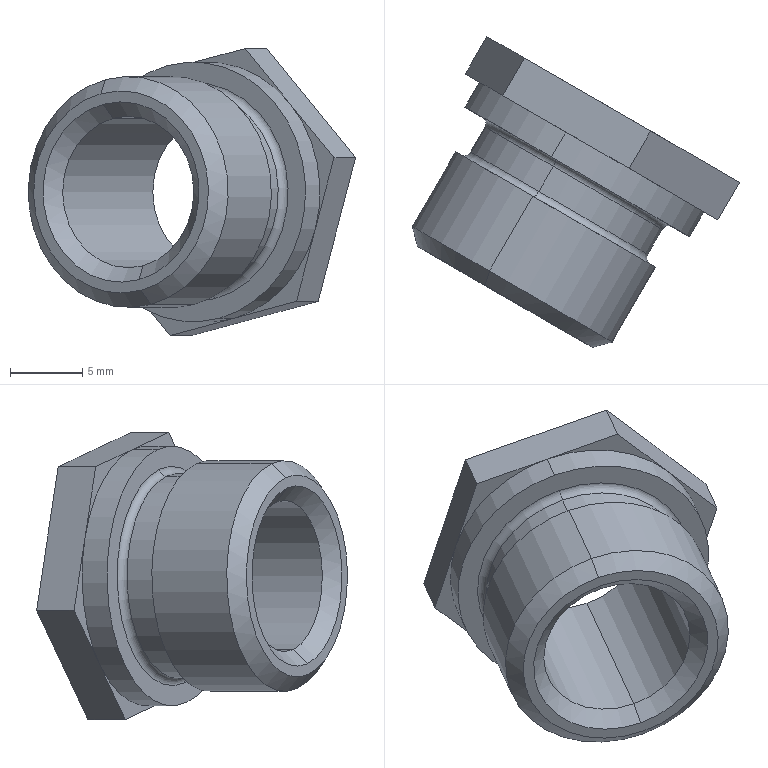Part | SolidWorks | features BaseBody 1 | 1 solid | 34 faces | box 22.69 x 21.549 x 19.899 mm | volume 1857 mm3 | plane 16 | cylinder 8 | cone 6 | torus 4 | commonest cylinder face diameters 10.5 x2 14.2 x2 16 x2 18 x2
STEP:
#1=CARTESIAN_POINT('',(323.84,252.406,-5.111));
#2=VERTEX_POINT('',#1);
#3=CARTESIAN_POINT('',(321.76,253.606,5.111));
#4=VERTEX_POINT('',#3);
#5=CARTESIAN_POINT('',(322.8,253.006,0.));
#6=DIRECTION('',(-0.5,-0.866,0.));
#7=DIRECTION('',(-0.198,0.1143,0.9735));
#8=AXIS2_PLACEMENT_3D('',#5,#6,#7);
#9=CIRCLE('',#8,5.25);
#10=EDGE_CURVE('',#2,#4,#9,.T.);
#11=ORIENTED_EDGE('',*,*,#10,.F.);
#12=CARTESIAN_POINT('',(323.538,251.425,-6.084));
#13=VERTEX_POINT('',#12);
#14=CARTESIAN_POINT('',(323.538,251.425,-6.084));
#15=DIRECTION('',(-0.2135,-0.6932,-0.6884));
#16=VECTOR('',#15,1000.);
#17=LINE('',#14,#16);
#18=EDGE_CURVE('',#2,#13,#17,.T.);
#19=ORIENTED_EDGE('',*,*,#18,.T.);
#20=CARTESIAN_POINT('',(321.062,252.854,6.084));
#21=VERTEX_POINT('',#20);
#22=CARTESIAN_POINT('',(322.3,252.14,0.));
#23=DIRECTION('',(0.5,0.866,0.));
#24=DIRECTION('',(-0.198,0.1143,0.9735));
#25=AXIS2_PLACEMENT_3D('',#22,#23,#24);
#26=CIRCLE('',#25,6.25);
#27=EDGE_CURVE('',#21,#13,#26,.T.);
#28=ORIENTED_EDGE('',*,*,#27,.F.);
#29=CARTESIAN_POINT('',(321.062,252.854,6.084));
#30=DIRECTION('',(-0.4936,-0.5315,0.6884));
#31=VECTOR('',#30,1000.);
#32=LINE('',#29,#31);
#33=EDGE_CURVE('',#4,#21,#32,.T.);
#34=ORIENTED_EDGE('',*,*,#33,.F.);
#35=EDGE_LOOP('',(#11,#19,#28,#34));
#36=FACE_OUTER_BOUND('',#35,.T.);
#37=CARTESIAN_POINT('',(322.3,252.14,0.));
#38=DIRECTION('',(-0.5,-0.866,0.));
#39=DIRECTION('',(-0.198,0.1143,0.9735));
#40=AXIS2_PLACEMENT_3D('',#37,#38,#39);
#41=CONICAL_SURFACE('',#40,6.25,0.7854);
#42=ADVANCED_FACE('',(#36),#41,.F.);
#43=CARTESIAN_POINT('',(328.01,264.431,5.111));
#44=VERTEX_POINT('',#43);
#45=CARTESIAN_POINT('',(330.09,263.231,-5.111));
#46=VERTEX_POINT('',#45);
#47=CARTESIAN_POINT('',(329.05,263.831,0.));
#48=DIRECTION('',(0.5,0.866,0.));
#49=DIRECTION('',(0.198,-0.1143,-0.9735));
#50=AXIS2_PLACEMENT_3D('',#47,#48,#49);
#51=CIRCLE('',#50,5.25);
#52=EDGE_CURVE('',#44,#46,#51,.T.);
#53=ORIENTED_EDGE('',*,*,#52,.F.);
#54=CARTESIAN_POINT('',(328.463,265.902,6.571));
#55=VERTEX_POINT('',#54);
#56=CARTESIAN_POINT('',(328.01,264.431,5.111));
#57=DIRECTION('',(0.2135,0.6932,0.6884));
#58=VECTOR('',#57,1000.);
#59=LINE('',#56,#58);
#60=EDGE_CURVE('',#44,#55,#59,.T.);
#61=ORIENTED_EDGE('',*,*,#60,.T.);
#62=CARTESIAN_POINT('',(331.137,264.358,-6.571));
#63=VERTEX_POINT('',#62);
#64=CARTESIAN_POINT('',(329.8,265.13,0.));
#65=DIRECTION('',(-0.5,-0.866,0.));
#66=DIRECTION('',(0.198,-0.1143,-0.9735));
#67=AXIS2_PLACEMENT_3D('',#64,#65,#66);
#68=CIRCLE('',#67,6.75);
#69=EDGE_CURVE('',#63,#55,#68,.T.);
#70=ORIENTED_EDGE('',*,*,#69,.F.);
#71=CARTESIAN_POINT('',(330.09,263.231,-5.111));
#72=DIRECTION('',(0.4936,0.5315,-0.6884));
#73=VECTOR('',#72,1000.);
#74=LINE('',#71,#73);
#75=EDGE_CURVE('',#46,#63,#74,.T.);
#76=ORIENTED_EDGE('',*,*,#75,.F.);
#77=EDGE_LOOP('',(#53,#61,#70,#76));
#78=FACE_OUTER_BOUND('',#77,.T.);
#79=CARTESIAN_POINT('',(329.05,263.831,0.));
#80=DIRECTION('',(0.5,0.866,0.));
#81=DIRECTION('',(0.198,-0.1143,-0.9735));
#82=AXIS2_PLACEMENT_3D('',#79,#80,#81);
#83=CONICAL_SURFACE('',#82,5.25,0.7854);
#84=ADVANCED_FACE('',(#78),#83,.F.);
#85=ORIENTED_EDGE('',*,*,#10,.T.);
#86=CARTESIAN_POINT('',(321.26,252.74,5.111));
#87=DIRECTION('',(0.5,0.866,0.));
#88=VECTOR('',#87,1000.);
#89=LINE('',#86,#88);
#90=EDGE_CURVE('',#4,#44,#89,.T.);
#91=ORIENTED_EDGE('',*,*,#90,.T.);
#92=ORIENTED_EDGE('',*,*,#52,.T.);
#93=CARTESIAN_POINT('',(323.34,251.54,-5.111));
#94=DIRECTION('',(0.5,0.866,0.));
#95=VECTOR('',#94,1000.);
#96=LINE('',#93,#95);
#97=EDGE_CURVE('',#2,#46,#96,.T.);
#98=ORIENTED_EDGE('',*,*,#97,.F.);
#99=EDGE_LOOP('',(#85,#91,#92,#98));
#100=FACE_OUTER_BOUND('',#99,.T.);
#101=CARTESIAN_POINT('',(322.3,252.14,0.));
#102=DIRECTION('',(0.5,0.866,0.));
#103=DIRECTION('',(0.198,-0.1143,-0.9735));
#104=AXIS2_PLACEMENT_3D('',#101,#102,#103);
#105=CYLINDRICAL_SURFACE('',#104,5.25);
#106=ADVANCED_FACE('',(#100),#105,.F.);
#107=CARTESIAN_POINT('',(327.305,257.333,-7.399));
#108=VERTEX_POINT('',#107);
#109=CARTESIAN_POINT('',(324.295,259.071,7.399));
#110=VERTEX_POINT('',#109);
#111=CARTESIAN_POINT('',(325.8,258.202,0.));
#112=DIRECTION('',(-0.5,-0.866,0.));
#113=DIRECTION('',(-0.198,0.1143,0.9735));
#114=AXIS2_PLACEMENT_3D('',#111,#112,#113);
#115=CIRCLE('',#114,7.6);
#116=EDGE_CURVE('',#108,#110,#115,.T.);
#117=ORIENTED_EDGE('',*,*,#116,.F.);
#118=CARTESIAN_POINT('',(327.456,257.823,-6.912));
#119=VERTEX_POINT('',#118);
#120=CARTESIAN_POINT('',(327.555,257.766,-7.399));
#121=DIRECTION('',(-0.8431,0.4868,-0.2286));
#122=DIRECTION('',(-0.5,-0.866,0.));
#123=AXIS2_PLACEMENT_3D('',#120,#121,#122);
#124=CIRCLE('',#123,0.5);
#125=EDGE_CURVE('',#108,#119,#124,.T.);
#126=ORIENTED_EDGE('',*,*,#125,.T.);
#127=CARTESIAN_POINT('',(324.644,259.447,6.912));
#128=VERTEX_POINT('',#127);
#129=CARTESIAN_POINT('',(326.05,258.635,0.));
#130=DIRECTION('',(0.5,0.866,0.));
#131=DIRECTION('',(-0.198,0.1143,0.9735));
#132=AXIS2_PLACEMENT_3D('',#129,#130,#131);
#133=CIRCLE('',#132,7.1);
#134=EDGE_CURVE('',#128,#119,#133,.T.);
#135=ORIENTED_EDGE('',*,*,#134,.F.);
#136=CARTESIAN_POINT('',(324.545,259.504,7.399));
#137=DIRECTION('',(0.8431,-0.4868,0.2286));
#138=DIRECTION('',(0.5,0.866,0.));
#139=AXIS2_PLACEMENT_3D('',#136,#137,#138);
#140=CIRCLE('',#139,0.5);
#141=EDGE_CURVE('',#110,#128,#140,.T.);
#142=ORIENTED_EDGE('',*,*,#141,.F.);
#143=EDGE_LOOP('',(#117,#126,#135,#142));
#144=FACE_OUTER_BOUND('',#143,.T.);
#145=CARTESIAN_POINT('',(326.05,258.635,0.));
#146=DIRECTION('',(-0.5,-0.866,0.));
#147=DIRECTION('',(-0.198,0.1143,0.9735));
#148=AXIS2_PLACEMENT_3D('',#145,#146,#147);
#149=TOROIDAL_SURFACE('',#148,7.6,0.5);
#150=ADVANCED_FACE('',(#144),#149,.F.);
#151=CARTESIAN_POINT('',(328.456,259.555,-6.912));
#152=VERTEX_POINT('',#151);
#153=CARTESIAN_POINT('',(325.644,261.179,6.912));
#154=VERTEX_POINT('',#153);
#155=CARTESIAN_POINT('',(327.05,260.367,0.));
#156=DIRECTION('',(-0.5,-0.866,0.));
#157=DIRECTION('',(-0.198,0.1143,0.9735));
#158=AXIS2_PLACEMENT_3D('',#155,#156,#157);
#159=CIRCLE('',#158,7.1);
#160=EDGE_CURVE('',#152,#154,#159,.T.);
#161=ORIENTED_EDGE('',*,*,#160,.F.);
#162=CARTESIAN_POINT('',(328.805,259.931,-7.399));
#163=VERTEX_POINT('',#162);
#164=CARTESIAN_POINT('',(328.555,259.498,-7.399));
#165=DIRECTION('',(-0.8431,0.4868,-0.2286));
#166=DIRECTION('',(-0.5,-0.866,0.));
#167=AXIS2_PLACEMENT_3D('',#164,#165,#166);
#168=CIRCLE('',#167,0.5);
#169=EDGE_CURVE('',#152,#163,#168,.T.);
#170=ORIENTED_EDGE('',*,*,#169,.T.);
#171=CARTESIAN_POINT('',(325.795,261.669,7.399));
#172=VERTEX_POINT('',#171);
#173=CARTESIAN_POINT('',(327.3,260.8,0.));
#174=DIRECTION('',(0.5,0.866,0.));
#175=DIRECTION('',(-0.198,0.1143,0.9735));
#176=AXIS2_PLACEMENT_3D('',#173,#174,#175);
#177=CIRCLE('',#176,7.6);
#178=EDGE_CURVE('',#172,#163,#177,.T.);
#179=ORIENTED_EDGE('',*,*,#178,.F.);
#180=CARTESIAN_POINT('',(325.545,261.236,7.399));
#181=DIRECTION('',(0.8431,-0.4868,0.2286));
#182=DIRECTION('',(0.5,0.866,0.));
#183=AXIS2_PLACEMENT_3D('',#180,#181,#182);
#184=CIRCLE('',#183,0.5);
#185=EDGE_CURVE('',#154,#172,#184,.T.);
#186=ORIENTED_EDGE('',*,*,#185,.F.);
#187=EDGE_LOOP('',(#161,#170,#179,#186));
#188=FACE_OUTER_BOUND('',#187,.T.);
#189=CARTESIAN_POINT('',(327.05,260.367,0.));
#190=DIRECTION('',(-0.5,-0.866,0.));
#191=DIRECTION('',(-0.198,0.1143,0.9735));
#192=AXIS2_PLACEMENT_3D('',#189,#190,#191);
#193=TOROIDAL_SURFACE('',#192,7.6,0.5);
#194=ADVANCED_FACE('',(#188),#193,.F.);
#195=CARTESIAN_POINT('',(320.914,252.94,6.815));
#196=VERTEX_POINT('',#195);
#197=CARTESIAN_POINT('',(323.686,251.34,-6.815));
#198=VERTEX_POINT('',#197);
#199=CARTESIAN_POINT('',(322.3,252.14,0.));
#200=DIRECTION('',(-0.5,-0.866,0.));
#201=DIRECTION('',(-0.198,0.1143,0.9735));
#202=AXIS2_PLACEMENT_3D('',#199,#200,#201);
#203=CIRCLE('',#202,7.);
#204=EDGE_CURVE('',#196,#198,#203,.T.);
#205=ORIENTED_EDGE('',*,*,#204,.F.);
#206=CARTESIAN_POINT('',(321.216,253.92,7.788));
#207=VERTEX_POINT('',#206);
#208=CARTESIAN_POINT('',(320.914,252.94,6.815));
#209=DIRECTION('',(0.2135,0.6932,0.6884));
#210=VECTOR('',#209,1000.);
#211=LINE('',#208,#210);
#212=EDGE_CURVE('',#196,#207,#211,.T.);
#213=ORIENTED_EDGE('',*,*,#212,.T.);
#214=CARTESIAN_POINT('',(324.384,252.091,-7.788));
#215=VERTEX_POINT('',#214);
#216=CARTESIAN_POINT('',(322.8,253.006,0.));
#217=DIRECTION('',(0.5,0.866,0.));
#218=DIRECTION('',(-0.198,0.1143,0.9735));
#219=AXIS2_PLACEMENT_3D('',#216,#217,#218);
#220=CIRCLE('',#219,8.);
#221=EDGE_CURVE('',#215,#207,#220,.T.);
#222=ORIENTED_EDGE('',*,*,#221,.F.);
#223=CARTESIAN_POINT('',(323.686,251.34,-6.815));
#224=DIRECTION('',(0.4936,0.5315,-0.6884));
#225=VECTOR('',#224,1000.);
#226=LINE('',#223,#225);
#227=EDGE_CURVE('',#198,#215,#226,.T.);
#228=ORIENTED_EDGE('',*,*,#227,.F.);
#229=EDGE_LOOP('',(#205,#213,#222,#228));
#230=FACE_OUTER_BOUND('',#229,.T.);
#231=CARTESIAN_POINT('',(322.3,252.14,0.));
#232=DIRECTION('',(0.5,0.866,0.));
#233=DIRECTION('',(0.198,-0.1143,-0.9735));
#234=AXIS2_PLACEMENT_3D('',#231,#232,#233);
#235=CONICAL_SURFACE('',#234,7.,0.7854);
#236=ADVANCED_FACE('',(#230),#235,.T.);
#237=ORIENTED_EDGE('',*,*,#221,.T.);
#238=CARTESIAN_POINT('',(324.216,259.116,7.788));
#239=VERTEX_POINT('',#238);
#240=CARTESIAN_POINT('',(306.402,228.262,7.788));
#241=DIRECTION('',(0.5,0.866,0.));
#242=VECTOR('',#241,1000.);
#243=LINE('',#240,#242);
#244=EDGE_CURVE('',#207,#239,#243,.T.);
#245=ORIENTED_EDGE('',*,*,#244,.T.);
#246=CARTESIAN_POINT('',(327.384,257.287,-7.788));
#247=VERTEX_POINT('',#246);
#248=CARTESIAN_POINT('',(325.8,258.202,0.));
#249=DIRECTION('',(-0.5,-0.866,0.));
#250=DIRECTION('',(-0.198,0.1143,0.9735));
#251=AXIS2_PLACEMENT_3D('',#248,#249,#250);
#252=CIRCLE('',#251,8.);
#253=EDGE_CURVE('',#239,#247,#252,.T.);
#254=ORIENTED_EDGE('',*,*,#253,.T.);
#255=CARTESIAN_POINT('',(309.57,226.433,-7.788));
#256=DIRECTION('',(0.5,0.866,0.));
#257=VECTOR('',#256,1000.);
#258=LINE('',#255,#257);
#259=EDGE_CURVE('',#215,#247,#258,.T.);
#260=ORIENTED_EDGE('',*,*,#259,.F.);
#261=EDGE_LOOP('',(#237,#245,#254,#260));
#262=FACE_OUTER_BOUND('',#261,.T.);
#263=CARTESIAN_POINT('',(307.986,227.348,0.));
#264=DIRECTION('',(0.5,0.866,0.));
#265=DIRECTION('',(0.198,-0.1143,-0.9735));
#266=AXIS2_PLACEMENT_3D('',#263,#264,#265);
#267=CYLINDRICAL_SURFACE('',#266,8.);
#268=ADVANCED_FACE('',(#262),#267,.T.);
#269=CARTESIAN_POINT('',(326.05,258.635,0.));
#270=DIRECTION('',(0.5,0.866,0.));
#271=DIRECTION('',(-0.198,0.1143,0.9735));
#272=AXIS2_PLACEMENT_3D('',#269,#270,#271);
#273=CIRCLE('',#272,7.1);
#274=EDGE_CURVE('',#119,#128,#273,.T.);
#275=ORIENTED_EDGE('',*,*,#274,.T.);
#276=CARTESIAN_POINT('',(324.394,259.014,6.912));
#277=DIRECTION('',(0.5,0.866,0.));
#278=VECTOR('',#277,1000.);
#279=LINE('',#276,#278);
#280=EDGE_CURVE('',#128,#154,#279,.T.);
#281=ORIENTED_EDGE('',*,*,#280,.T.);
#282=CARTESIAN_POINT('',(327.05,260.367,0.));
#283=DIRECTION('',(-0.5,-0.866,0.));
#284=DIRECTION('',(-0.198,0.1143,0.9735));
#285=AXIS2_PLACEMENT_3D('',#282,#283,#284);
#286=CIRCLE('',#285,7.1);
#287=EDGE_CURVE('',#154,#152,#286,.T.);
#288=ORIENTED_EDGE('',*,*,#287,.T.);
#289=CARTESIAN_POINT('',(327.206,257.39,-6.912));
#290=DIRECTION('',(0.5,0.866,0.));
#291=VECTOR('',#290,1000.);
#292=LINE('',#289,#291);
#293=EDGE_CURVE('',#119,#152,#292,.T.);
#294=ORIENTED_EDGE('',*,*,#293,.F.);
#295=EDGE_LOOP('',(#275,#281,#288,#294));
#296=FACE_OUTER_BOUND('',#295,.T.);
#297=CARTESIAN_POINT('',(325.8,258.202,0.));
#298=DIRECTION('',(0.5,0.866,0.));
#299=DIRECTION('',(0.198,-0.1143,-0.9735));
#300=AXIS2_PLACEMENT_3D('',#297,#298,#299);
#301=CYLINDRICAL_SURFACE('',#300,7.1);
#302=ADVANCED_FACE('',(#296),#301,.T.);
#303=CARTESIAN_POINT('',(325.518,261.829,8.762));
#304=VERTEX_POINT('',#303);
#305=CARTESIAN_POINT('',(329.082,259.771,-8.762));
#306=VERTEX_POINT('',#305);
#307=CARTESIAN_POINT('',(327.3,260.8,0.));
#308=DIRECTION('',(-0.5,-0.866,0.));
#309=DIRECTION('',(-0.198,0.1143,0.9735));
#310=AXIS2_PLACEMENT_3D('',#307,#308,#309);
#311=CIRCLE('',#310,9.);
#312=EDGE_CURVE('',#304,#306,#311,.T.);
#313=ORIENTED_EDGE('',*,*,#312,.F.);
#314=CARTESIAN_POINT('',(326.518,263.561,8.762));
#315=VERTEX_POINT('',#314);
#316=CARTESIAN_POINT('',(325.518,261.829,8.762));
#317=DIRECTION('',(0.5,0.866,0.));
#318=VECTOR('',#317,1000.);
#319=LINE('',#316,#318);
#320=EDGE_CURVE('',#304,#315,#319,.T.);
#321=ORIENTED_EDGE('',*,*,#320,.T.);
#322=CARTESIAN_POINT('',(320.838,266.84,2.599));
#323=VERTEX_POINT('',#322);
#324=CARTESIAN_POINT('',(328.3,262.532,0.));
#325=DIRECTION('',(-0.5,-0.866,0.));
#326=DIRECTION('',(-0.198,0.1143,0.9735));
#327=AXIS2_PLACEMENT_3D('',#324,#325,#326);
#328=CIRCLE('',#327,9.);
#329=EDGE_CURVE('',#315,#323,#328,.T.);
#330=ORIENTED_EDGE('',*,*,#329,.T.);
#331=CARTESIAN_POINT('',(322.62,265.812,-6.163));
#332=VERTEX_POINT('',#331);
#333=CARTESIAN_POINT('',(328.3,262.532,0.));
#334=DIRECTION('',(-0.5,-0.866,0.));
#335=DIRECTION('',(-0.198,0.1143,0.9735));
#336=AXIS2_PLACEMENT_3D('',#333,#334,#335);
#337=CIRCLE('',#336,9.);
#338=EDGE_CURVE('',#323,#332,#337,.T.);
#339=ORIENTED_EDGE('',*,*,#338,.T.);
#340=CARTESIAN_POINT('',(330.082,261.503,-8.762));
#341=VERTEX_POINT('',#340);
#342=CARTESIAN_POINT('',(328.3,262.532,0.));
#343=DIRECTION('',(-0.5,-0.866,0.));
#344=DIRECTION('',(-0.198,0.1143,0.9735));
#345=AXIS2_PLACEMENT_3D('',#342,#343,#344);
#346=CIRCLE('',#345,9.);
#347=EDGE_CURVE('',#332,#341,#346,.T.);
#348=ORIENTED_EDGE('',*,*,#347,.T.);
#349=CARTESIAN_POINT('',(329.082,259.771,-8.762));
#350=DIRECTION('',(0.5,0.866,0.));
#351=VECTOR('',#350,1000.);
#352=LINE('',#349,#351);
#353=EDGE_CURVE('',#306,#341,#352,.T.);
#354=ORIENTED_EDGE('',*,*,#353,.F.);
#355=EDGE_LOOP('',(#313,#321,#330,#339,#348,#354));
#356=FACE_OUTER_BOUND('',#355,.T.);
#357=CARTESIAN_POINT('',(327.3,260.8,0.));
#358=DIRECTION('',(0.5,0.866,0.));
#359=DIRECTION('',(0.198,-0.1143,-0.9735));
#360=AXIS2_PLACEMENT_3D('',#357,#358,#359);
#361=CYLINDRICAL_SURFACE('',#360,9.);
#362=ADVANCED_FACE('',(#356),#361,.T.);
#363=ORIENTED_EDGE('',*,*,#178,.T.);
#364=CARTESIAN_POINT('',(327.3,260.8,0.));
#365=DIRECTION('',(0.5,0.866,0.));
#366=DIRECTION('',(-0.198,0.1143,0.9735));
#367=AXIS2_PLACEMENT_3D('',#364,#365,#366);
#368=CIRCLE('',#367,7.6);
#369=EDGE_CURVE('',#163,#172,#368,.T.);
#370=ORIENTED_EDGE('',*,*,#369,.T.);
#371=EDGE_LOOP('',(#363,#370));
#372=FACE_BOUND('',#371,.T.);
#373=CARTESIAN_POINT('',(327.3,260.8,0.));
#374=DIRECTION('',(-0.5,-0.866,0.));
#375=DIRECTION('',(-0.198,0.1143,0.9735));
#376=AXIS2_PLACEMENT_3D('',#373,#374,#375);
#377=CIRCLE('',#376,9.);
#378=EDGE_CURVE('',#306,#304,#377,.T.);
#379=ORIENTED_EDGE('',*,*,#378,.T.);
#380=ORIENTED_EDGE('',*,*,#312,.T.);
#381=EDGE_LOOP('',(#379,#380));
#382=FACE_OUTER_BOUND('',#381,.T.);
#383=CARTESIAN_POINT('',(327.3,260.8,0.));
#384=DIRECTION('',(-0.5,-0.866,0.));
#385=DIRECTION('',(-0.198,0.1143,0.9735));
#386=AXIS2_PLACEMENT_3D('',#383,#384,#385);
#387=PLANE('',#386);
#388=ADVANCED_FACE('',(#372,#382),#387,.T.);
#389=ORIENTED_EDGE('',*,*,#329,.F.);
#390=CARTESIAN_POINT('',(322.137,266.09,7.574));
#391=VERTEX_POINT('',#390);
#392=CARTESIAN_POINT('',(330.899,261.032,9.95));
#393=DIRECTION('',(-0.8431,0.4868,-0.2286));
#394=VECTOR('',#393,1000.);
#395=LINE('',#392,#394);
#396=EDGE_CURVE('',#315,#391,#395,.T.);
#397=ORIENTED_EDGE('',*,*,#396,.T.);
#398=CARTESIAN_POINT('',(322.137,266.09,7.574));
#399=DIRECTION('',(-0.2501,0.1444,-0.9574));
#400=VECTOR('',#399,1000.);
#401=LINE('',#398,#400);
#402=EDGE_CURVE('',#391,#323,#401,.T.);
#403=ORIENTED_EDGE('',*,*,#402,.T.);
#404=EDGE_LOOP('',(#389,#397,#403));
#405=FACE_OUTER_BOUND('',#404,.T.);
#406=CARTESIAN_POINT('',(319.538,267.591,-2.376));
#407=DIRECTION('',(0.5,0.866,0.));
#408=DIRECTION('',(0.198,-0.1143,-0.9735));
#409=AXIS2_PLACEMENT_3D('',#406,#407,#408);
#410=PLANE('',#409);
#411=ADVANCED_FACE('',(#405),#410,.F.);
#412=ORIENTED_EDGE('',*,*,#338,.F.);
#413=CARTESIAN_POINT('',(319.538,267.591,-2.376));
#414=VERTEX_POINT('',#413);
#415=CARTESIAN_POINT('',(322.137,266.09,7.574));
#416=DIRECTION('',(-0.2501,0.1444,-0.9574));
#417=VECTOR('',#416,1000.);
#418=LINE('',#415,#417);
#419=EDGE_CURVE('',#323,#414,#418,.T.);
#420=ORIENTED_EDGE('',*,*,#419,.T.);
#421=CARTESIAN_POINT('',(325.701,264.032,-9.95));
#422=DIRECTION('',(0.593,-0.3424,-0.7288));
#423=VECTOR('',#422,1000.);
#424=LINE('',#421,#423);
#425=EDGE_CURVE('',#414,#332,#424,.T.);
#426=ORIENTED_EDGE('',*,*,#425,.T.);
#427=EDGE_LOOP('',(#412,#420,#426));
#428=FACE_OUTER_BOUND('',#427,.T.);
#429=CARTESIAN_POINT('',(319.538,267.591,-2.376));
#430=DIRECTION('',(0.5,0.866,0.));
#431=DIRECTION('',(0.198,-0.1143,-0.9735));
#432=AXIS2_PLACEMENT_3D('',#429,#430,#431);
#433=PLANE('',#432);
#434=ADVANCED_FACE('',(#428),#433,.F.);
#435=ORIENTED_EDGE('',*,*,#347,.F.);
#436=CARTESIAN_POINT('',(325.701,264.032,-9.95));
#437=VERTEX_POINT('',#436);
#438=CARTESIAN_POINT('',(325.701,264.032,-9.95));
#439=DIRECTION('',(0.593,-0.3424,-0.7288));
#440=VECTOR('',#439,1000.);
#441=LINE('',#438,#440);
#442=EDGE_CURVE('',#332,#437,#441,.T.);
#443=ORIENTED_EDGE('',*,*,#442,.T.);
#444=CARTESIAN_POINT('',(334.463,258.974,-7.574));
#445=DIRECTION('',(0.8431,-0.4868,0.2286));
#446=VECTOR('',#445,1000.);
#447=LINE('',#444,#446);
#448=EDGE_CURVE('',#437,#341,#447,.T.);
#449=ORIENTED_EDGE('',*,*,#448,.T.);
#450=EDGE_LOOP('',(#435,#443,#449));
#451=FACE_OUTER_BOUND('',#450,.T.);
#452=CARTESIAN_POINT('',(319.538,267.591,-2.376));
#453=DIRECTION('',(0.5,0.866,0.));
#454=DIRECTION('',(0.198,-0.1143,-0.9735));
#455=AXIS2_PLACEMENT_3D('',#452,#453,#454);
#456=PLANE('',#455);
#457=ADVANCED_FACE('',(#451),#456,.F.);
#458=CARTESIAN_POINT('',(335.762,258.224,-2.599));
#459=VERTEX_POINT('',#458);
#460=CARTESIAN_POINT('',(328.3,262.532,0.));
#461=DIRECTION('',(-0.5,-0.866,0.));
#462=DIRECTION('',(-0.198,0.1143,0.9735));
#463=AXIS2_PLACEMENT_3D('',#460,#461,#462);
#464=CIRCLE('',#463,9.);
#465=EDGE_CURVE('',#341,#459,#464,.T.);
#466=ORIENTED_EDGE('',*,*,#465,.F.);
#467=CARTESIAN_POINT('',(334.463,258.974,-7.574));
#468=VERTEX_POINT('',#467);
#469=CARTESIAN_POINT('',(334.463,258.974,-7.574));
#470=DIRECTION('',(0.8431,-0.4868,0.2286));
#471=VECTOR('',#470,1000.);
#472=LINE('',#469,#471);
#473=EDGE_CURVE('',#341,#468,#472,.T.);
#474=ORIENTED_EDGE('',*,*,#473,.T.);
#475=CARTESIAN_POINT('',(334.463,258.974,-7.574));
#476=DIRECTION('',(0.2501,-0.1444,0.9574));
#477=VECTOR('',#476,1000.);
#478=LINE('',#475,#477);
#479=EDGE_CURVE('',#468,#459,#478,.T.);
#480=ORIENTED_EDGE('',*,*,#479,.T.);
#481=EDGE_LOOP('',(#466,#474,#480));
#482=FACE_OUTER_BOUND('',#481,.T.);
#483=CARTESIAN_POINT('',(319.538,267.591,-2.376));
#484=DIRECTION('',(0.5,0.866,0.));
#485=DIRECTION('',(0.198,-0.1143,-0.9735));
#486=AXIS2_PLACEMENT_3D('',#483,#484,#485);
#487=PLANE('',#486);
#488=ADVANCED_FACE('',(#482),#487,.F.);
#489=CARTESIAN_POINT('',(333.98,259.253,6.163));
#490=VERTEX_POINT('',#489);
#491=CARTESIAN_POINT('',(328.3,262.532,0.));
#492=DIRECTION('',(-0.5,-0.866,0.));
#493=DIRECTION('',(-0.198,0.1143,0.9735));
#494=AXIS2_PLACEMENT_3D('',#491,#492,#493);
#495=CIRCLE('',#494,9.);
#496=EDGE_CURVE('',#459,#490,#495,.T.);
#497=ORIENTED_EDGE('',*,*,#496,.F.);
#498=CARTESIAN_POINT('',(337.062,257.474,2.376));
#499=VERTEX_POINT('',#498);
#500=CARTESIAN_POINT('',(334.463,258.974,-7.574));
#501=DIRECTION('',(0.2501,-0.1444,0.9574));
#502=VECTOR('',#501,1000.);
#503=LINE('',#500,#502);
#504=EDGE_CURVE('',#459,#499,#503,.T.);
#505=ORIENTED_EDGE('',*,*,#504,.T.);
#506=CARTESIAN_POINT('',(330.899,261.032,9.95));
#507=DIRECTION('',(-0.593,0.3424,0.7288));
#508=VECTOR('',#507,1000.);
#509=LINE('',#506,#508);
#510=EDGE_CURVE('',#499,#490,#509,.T.);
#511=ORIENTED_EDGE('',*,*,#510,.T.);
#512=EDGE_LOOP('',(#497,#505,#511));
#513=FACE_OUTER_BOUND('',#512,.T.);
#514=CARTESIAN_POINT('',(319.538,267.591,-2.376));
#515=DIRECTION('',(0.5,0.866,0.));
#516=DIRECTION('',(0.198,-0.1143,-0.9735));
#517=AXIS2_PLACEMENT_3D('',#514,#515,#516);
#518=PLANE('',#517);
#519=ADVANCED_FACE('',(#513),#518,.F.);
#520=CARTESIAN_POINT('',(328.3,262.532,0.));
#521=DIRECTION('',(-0.5,-0.866,0.));
#522=DIRECTION('',(-0.198,0.1143,0.9735));
#523=AXIS2_PLACEMENT_3D('',#520,#521,#522);
#524=CIRCLE('',#523,9.);
#525=EDGE_CURVE('',#490,#315,#524,.T.);
#526=ORIENTED_EDGE('',*,*,#525,.F.);
#527=CARTESIAN_POINT('',(330.899,261.032,9.95));
#528=VERTEX_POINT('',#527);
#529=CARTESIAN_POINT('',(330.899,261.032,9.95));
#530=DIRECTION('',(-0.593,0.3424,0.7288));
#531=VECTOR('',#530,1000.);
#532=LINE('',#529,#531);
#533=EDGE_CURVE('',#490,#528,#532,.T.);
#534=ORIENTED_EDGE('',*,*,#533,.T.);
#535=CARTESIAN_POINT('',(330.899,261.032,9.95));
#536=DIRECTION('',(-0.8431,0.4868,-0.2286));
#537=VECTOR('',#536,1000.);
#538=LINE('',#535,#537);
#539=EDGE_CURVE('',#528,#315,#538,.T.);
#540=ORIENTED_EDGE('',*,*,#539,.T.);
#541=EDGE_LOOP('',(#526,#534,#540));
#542=FACE_OUTER_BOUND('',#541,.T.);
#543=CARTESIAN_POINT('',(319.538,267.591,-2.376));
#544=DIRECTION('',(0.5,0.866,0.));
#545=DIRECTION('',(0.198,-0.1143,-0.9735));
#546=AXIS2_PLACEMENT_3D('',#543,#544,#545);
#547=PLANE('',#546);
#548=ADVANCED_FACE('',(#542),#547,.F.);
#549=CARTESIAN_POINT('',(323.637,268.688,7.574));
#550=VERTEX_POINT('',#549);
#551=CARTESIAN_POINT('',(321.038,270.189,-2.376));
#552=VERTEX_POINT('',#551);
#553=CARTESIAN_POINT('',(323.637,268.688,7.574));
#554=DIRECTION('',(-0.2501,0.1444,-0.9574));
#555=VECTOR('',#554,1000.);
#556=LINE('',#553,#555);
#557=EDGE_CURVE('',#550,#552,#556,.T.);
#558=ORIENTED_EDGE('',*,*,#557,.T.);
#559=CARTESIAN_POINT('',(319.538,267.591,-2.376));
#560=DIRECTION('',(0.5,0.866,0.));
#561=VECTOR('',#560,1000.);
#562=LINE('',#559,#561);
#563=EDGE_CURVE('',#414,#552,#562,.T.);
#564=ORIENTED_EDGE('',*,*,#563,.F.);
#565=ORIENTED_EDGE('',*,*,#419,.F.);
#566=ORIENTED_EDGE('',*,*,#402,.F.);
#567=CARTESIAN_POINT('',(322.137,266.09,7.574));
#568=DIRECTION('',(0.5,0.866,0.));
#569=VECTOR('',#568,1000.);
#570=LINE('',#567,#569);
#571=EDGE_CURVE('',#391,#550,#570,.T.);
#572=ORIENTED_EDGE('',*,*,#571,.T.);
#573=EDGE_LOOP('',(#558,#564,#565,#566,#572));
#574=FACE_OUTER_BOUND('',#573,.T.);
#575=CARTESIAN_POINT('',(322.137,266.09,7.574));
#576=DIRECTION('',(0.8291,-0.4787,-0.2887));
#577=DIRECTION('',(0.2501,-0.1444,0.9574));
#578=AXIS2_PLACEMENT_3D('',#575,#576,#577);
#579=PLANE('',#578);
#580=ADVANCED_FACE('',(#574),#579,.F.);
#581=CARTESIAN_POINT('',(327.201,266.631,-9.95));
#582=VERTEX_POINT('',#581);
#583=CARTESIAN_POINT('',(327.201,266.631,-9.95));
#584=DIRECTION('',(0.593,-0.3424,-0.7288));
#585=VECTOR('',#584,1000.);
#586=LINE('',#583,#585);
#587=EDGE_CURVE('',#552,#582,#586,.T.);
#588=ORIENTED_EDGE('',*,*,#587,.T.);
#589=CARTESIAN_POINT('',(325.701,264.032,-9.95));
#590=DIRECTION('',(0.5,0.866,0.));
#591=VECTOR('',#590,1000.);
#592=LINE('',#589,#591);
#593=EDGE_CURVE('',#437,#582,#592,.T.);
#594=ORIENTED_EDGE('',*,*,#593,.F.);
#595=ORIENTED_EDGE('',*,*,#442,.F.);
#596=ORIENTED_EDGE('',*,*,#425,.F.);
#597=ORIENTED_EDGE('',*,*,#563,.T.);
#598=EDGE_LOOP('',(#588,#594,#595,#596,#597));
#599=FACE_OUTER_BOUND('',#598,.T.);
#600=CARTESIAN_POINT('',(325.701,264.032,-9.95));
#601=DIRECTION('',(0.6311,-0.3644,0.6848));
#602=DIRECTION('',(-0.593,0.3424,0.7288));
#603=AXIS2_PLACEMENT_3D('',#600,#601,#602);
#604=PLANE('',#603);
#605=ADVANCED_FACE('',(#599),#604,.F.);
#606=CARTESIAN_POINT('',(335.963,261.572,-7.574));
#607=VERTEX_POINT('',#606);
#608=CARTESIAN_POINT('',(335.963,261.572,-7.574));
#609=DIRECTION('',(0.8431,-0.4868,0.2286));
#610=VECTOR('',#609,1000.);
#611=LINE('',#608,#610);
#612=EDGE_CURVE('',#582,#607,#611,.T.);
#613=ORIENTED_EDGE('',*,*,#612,.T.);
#614=CARTESIAN_POINT('',(334.463,258.974,-7.574));
#615=DIRECTION('',(0.5,0.866,0.));
#616=VECTOR('',#615,1000.);
#617=LINE('',#614,#616);
#618=EDGE_CURVE('',#468,#607,#617,.T.);
#619=ORIENTED_EDGE('',*,*,#618,.F.);
#620=ORIENTED_EDGE('',*,*,#473,.F.);
#621=ORIENTED_EDGE('',*,*,#448,.F.);
#622=ORIENTED_EDGE('',*,*,#593,.T.);
#623=EDGE_LOOP('',(#613,#619,#620,#621,#622));
#624=FACE_OUTER_BOUND('',#623,.T.);
#625=CARTESIAN_POINT('',(334.463,258.974,-7.574));
#626=DIRECTION('',(-0.198,0.1143,0.9735));
#627=DIRECTION('',(0.5,0.866,0.));
#628=AXIS2_PLACEMENT_3D('',#625,#626,#627);
#629=PLANE('',#628);
#630=ADVANCED_FACE('',(#624),#629,.F.);
#631=CARTESIAN_POINT('',(338.562,260.072,2.376));
#632=VERTEX_POINT('',#631);
#633=CARTESIAN_POINT('',(335.963,261.572,-7.574));
#634=DIRECTION('',(0.2501,-0.1444,0.9574));
#635=VECTOR('',#634,1000.);
#636=LINE('',#633,#635);
#637=EDGE_CURVE('',#607,#632,#636,.T.);
#638=ORIENTED_EDGE('',*,*,#637,.T.);
#639=CARTESIAN_POINT('',(337.062,257.474,2.376));
#640=DIRECTION('',(0.5,0.866,0.));
#641=VECTOR('',#640,1000.);
#642=LINE('',#639,#641);
#643=EDGE_CURVE('',#499,#632,#642,.T.);
#644=ORIENTED_EDGE('',*,*,#643,.F.);
#645=ORIENTED_EDGE('',*,*,#504,.F.);
#646=ORIENTED_EDGE('',*,*,#479,.F.);
#647=ORIENTED_EDGE('',*,*,#618,.T.);
#648=EDGE_LOOP('',(#638,#644,#645,#646,#647));
#649=FACE_OUTER_BOUND('',#648,.T.);
#650=CARTESIAN_POINT('',(334.463,258.974,-7.574));
#651=DIRECTION('',(-0.8291,0.4787,0.2887));
#652=DIRECTION('',(-0.2501,0.1444,-0.9574));
#653=AXIS2_PLACEMENT_3D('',#650,#651,#652);
#654=PLANE('',#653);
#655=ADVANCED_FACE('',(#649),#654,.F.);
#656=CARTESIAN_POINT('',(332.399,263.63,9.95));
#657=VERTEX_POINT('',#656);
#658=CARTESIAN_POINT('',(332.399,263.63,9.95));
#659=DIRECTION('',(-0.593,0.3424,0.7288));
#660=VECTOR('',#659,1000.);
#661=LINE('',#658,#660);
#662=EDGE_CURVE('',#632,#657,#661,.T.);
#663=ORIENTED_EDGE('',*,*,#662,.T.);
#664=CARTESIAN_POINT('',(330.899,261.032,9.95));
#665=DIRECTION('',(0.5,0.866,0.));
#666=VECTOR('',#665,1000.);
#667=LINE('',#664,#666);
#668=EDGE_CURVE('',#528,#657,#667,.T.);
#669=ORIENTED_EDGE('',*,*,#668,.F.);
#670=ORIENTED_EDGE('',*,*,#533,.F.);
#671=ORIENTED_EDGE('',*,*,#510,.F.);
#672=ORIENTED_EDGE('',*,*,#643,.T.);
#673=EDGE_LOOP('',(#663,#669,#670,#671,#672));
#674=FACE_OUTER_BOUND('',#673,.T.);
#675=CARTESIAN_POINT('',(330.899,261.032,9.95));
#676=DIRECTION('',(-0.6311,0.3644,-0.6848));
#677=DIRECTION('',(0.593,-0.3424,-0.7288));
#678=AXIS2_PLACEMENT_3D('',#675,#676,#677);
#679=PLANE('',#678);
#680=ADVANCED_FACE('',(#674),#679,.F.);
#681=CARTESIAN_POINT('',(332.399,263.63,9.95));
#682=DIRECTION('',(-0.8431,0.4868,-0.2286));
#683=VECTOR('',#682,1000.);
#684=LINE('',#681,#683);
#685=EDGE_CURVE('',#657,#550,#684,.T.);
#686=ORIENTED_EDGE('',*,*,#685,.T.);
#687=ORIENTED_EDGE('',*,*,#571,.F.);
#688=ORIENTED_EDGE('',*,*,#396,.F.);
#689=ORIENTED_EDGE('',*,*,#539,.F.);
#690=ORIENTED_EDGE('',*,*,#668,.T.);
#691=EDGE_LOOP('',(#686,#687,#688,#689,#690));
#692=FACE_OUTER_BOUND('',#691,.T.);
#693=CARTESIAN_POINT('',(330.899,261.032,9.95));
#694=DIRECTION('',(0.198,-0.1143,-0.9735));
#695=DIRECTION('',(-0.5,-0.866,0.));
#696=AXIS2_PLACEMENT_3D('',#693,#694,#695);
#697=PLANE('',#696);
#698=ADVANCED_FACE('',(#692),#697,.F.);
#699=ORIENTED_EDGE('',*,*,#69,.T.);
#700=CARTESIAN_POINT('',(329.8,265.13,0.));
#701=DIRECTION('',(-0.5,-0.866,0.));
#702=DIRECTION('',(0.198,-0.1143,-0.9735));
#703=AXIS2_PLACEMENT_3D('',#700,#701,#702);
#704=CIRCLE('',#703,6.75);
#705=EDGE_CURVE('',#55,#63,#704,.T.);
#706=ORIENTED_EDGE('',*,*,#705,.T.);
#707=EDGE_LOOP('',(#699,#706));
#708=FACE_BOUND('',#707,.T.);
#709=ORIENTED_EDGE('',*,*,#557,.F.);
#710=ORIENTED_EDGE('',*,*,#685,.F.);
#711=ORIENTED_EDGE('',*,*,#662,.F.);
#712=ORIENTED_EDGE('',*,*,#637,.F.);
#713=ORIENTED_EDGE('',*,*,#612,.F.);
#714=ORIENTED_EDGE('',*,*,#587,.F.);
#715=EDGE_LOOP('',(#709,#710,#711,#712,#713,#714));
#716=FACE_OUTER_BOUND('',#715,.T.);
#717=CARTESIAN_POINT('',(321.038,270.189,-2.376));
#718=DIRECTION('',(0.5,0.866,0.));
#719=DIRECTION('',(0.198,-0.1143,-0.9735));
#720=AXIS2_PLACEMENT_3D('',#717,#718,#719);
#721=PLANE('',#720);
#722=ADVANCED_FACE('',(#708,#716),#721,.T.);
#723=ORIENTED_EDGE('',*,*,#320,.F.);
#724=ORIENTED_EDGE('',*,*,#378,.F.);
#725=ORIENTED_EDGE('',*,*,#353,.T.);
#726=ORIENTED_EDGE('',*,*,#465,.T.);
#727=ORIENTED_EDGE('',*,*,#496,.T.);
#728=ORIENTED_EDGE('',*,*,#525,.T.);
#729=EDGE_LOOP('',(#723,#724,#725,#726,#727,#728));
#730=FACE_OUTER_BOUND('',#729,.T.);
#731=CARTESIAN_POINT('',(327.3,260.8,0.));
#732=DIRECTION('',(0.5,0.866,0.));
#733=DIRECTION('',(0.198,-0.1143,-0.9735));
#734=AXIS2_PLACEMENT_3D('',#731,#732,#733);
#735=CYLINDRICAL_SURFACE('',#734,9.);
#736=ADVANCED_FACE('',(#730),#735,.T.);
#737=ORIENTED_EDGE('',*,*,#280,.F.);
#738=ORIENTED_EDGE('',*,*,#134,.T.);
#739=ORIENTED_EDGE('',*,*,#293,.T.);
#740=ORIENTED_EDGE('',*,*,#160,.T.);
#741=EDGE_LOOP('',(#737,#738,#739,#740));
#742=FACE_OUTER_BOUND('',#741,.T.);
#743=CARTESIAN_POINT('',(325.8,258.202,0.));
#744=DIRECTION('',(0.5,0.866,0.));
#745=DIRECTION('',(0.198,-0.1143,-0.9735));
#746=AXIS2_PLACEMENT_3D('',#743,#744,#745);
#747=CYLINDRICAL_SURFACE('',#746,7.1);
#748=ADVANCED_FACE('',(#742),#747,.T.);
#749=CARTESIAN_POINT('',(325.8,258.202,0.));
#750=DIRECTION('',(-0.5,-0.866,0.));
#751=DIRECTION('',(-0.198,0.1143,0.9735));
#752=AXIS2_PLACEMENT_3D('',#749,#750,#751);
#753=CIRCLE('',#752,7.6);
#754=EDGE_CURVE('',#110,#108,#753,.T.);
#755=ORIENTED_EDGE('',*,*,#754,.T.);
#756=ORIENTED_EDGE('',*,*,#116,.T.);
#757=EDGE_LOOP('',(#755,#756));
#758=FACE_BOUND('',#757,.T.);
#759=CARTESIAN_POINT('',(325.8,258.202,0.));
#760=DIRECTION('',(-0.5,-0.866,0.));
#761=DIRECTION('',(-0.198,0.1143,0.9735));
#762=AXIS2_PLACEMENT_3D('',#759,#760,#761);
#763=CIRCLE('',#762,8.);
#764=EDGE_CURVE('',#247,#239,#763,.T.);
#765=ORIENTED_EDGE('',*,*,#764,.F.);
#766=ORIENTED_EDGE('',*,*,#253,.F.);
#767=EDGE_LOOP('',(#765,#766));
#768=FACE_OUTER_BOUND('',#767,.T.);
#769=CARTESIAN_POINT('',(325.8,258.202,0.));
#770=DIRECTION('',(-0.5,-0.866,0.));
#771=DIRECTION('',(-0.198,0.1143,0.9735));
#772=AXIS2_PLACEMENT_3D('',#769,#770,#771);
#773=PLANE('',#772);
#774=ADVANCED_FACE('',(#758,#768),#773,.F.);
#775=ORIENTED_EDGE('',*,*,#244,.F.);
#776=CARTESIAN_POINT('',(322.8,253.006,0.));
#777=DIRECTION('',(0.5,0.866,0.));
#778=DIRECTION('',(-0.198,0.1143,0.9735));
#779=AXIS2_PLACEMENT_3D('',#776,#777,#778);
#780=CIRCLE('',#779,8.);
#781=EDGE_CURVE('',#207,#215,#780,.T.);
#782=ORIENTED_EDGE('',*,*,#781,.T.);
#783=ORIENTED_EDGE('',*,*,#259,.T.);
#784=ORIENTED_EDGE('',*,*,#764,.T.);
#785=EDGE_LOOP('',(#775,#782,#783,#784));
#786=FACE_OUTER_BOUND('',#785,.T.);
#787=CARTESIAN_POINT('',(307.986,227.348,0.));
#788=DIRECTION('',(0.5,0.866,0.));
#789=DIRECTION('',(0.198,-0.1143,-0.9735));
#790=AXIS2_PLACEMENT_3D('',#787,#788,#789);
#791=CYLINDRICAL_SURFACE('',#790,8.);
#792=ADVANCED_FACE('',(#786),#791,.T.);
#793=ORIENTED_EDGE('',*,*,#27,.T.);
#794=CARTESIAN_POINT('',(322.3,252.14,0.));
#795=DIRECTION('',(0.5,0.866,0.));
#796=DIRECTION('',(-0.198,0.1143,0.9735));
#797=AXIS2_PLACEMENT_3D('',#794,#795,#796);
#798=CIRCLE('',#797,6.25);
#799=EDGE_CURVE('',#13,#21,#798,.T.);
#800=ORIENTED_EDGE('',*,*,#799,.T.);
#801=EDGE_LOOP('',(#793,#800));
#802=FACE_BOUND('',#801,.T.);
#803=CARTESIAN_POINT('',(322.3,252.14,0.));
#804=DIRECTION('',(-0.5,-0.866,0.));
#805=DIRECTION('',(-0.198,0.1143,0.9735));
#806=AXIS2_PLACEMENT_3D('',#803,#804,#805);
#807=CIRCLE('',#806,7.);
#808=EDGE_CURVE('',#198,#196,#807,.T.);
#809=ORIENTED_EDGE('',*,*,#808,.T.);
#810=ORIENTED_EDGE('',*,*,#204,.T.);
#811=EDGE_LOOP('',(#809,#810));
#812=FACE_OUTER_BOUND('',#811,.T.);
#813=CARTESIAN_POINT('',(322.3,252.14,0.));
#814=DIRECTION('',(-0.5,-0.866,0.));
#815=DIRECTION('',(-0.198,0.1143,0.9735));
#816=AXIS2_PLACEMENT_3D('',#813,#814,#815);
#817=PLANE('',#816);
#818=ADVANCED_FACE('',(#802,#812),#817,.T.);
#819=ORIENTED_EDGE('',*,*,#212,.F.);
#820=ORIENTED_EDGE('',*,*,#808,.F.);
#821=ORIENTED_EDGE('',*,*,#227,.T.);
#822=ORIENTED_EDGE('',*,*,#781,.F.);
#823=EDGE_LOOP('',(#819,#820,#821,#822));
#824=FACE_OUTER_BOUND('',#823,.T.);
#825=CARTESIAN_POINT('',(322.3,252.14,0.));
#826=DIRECTION('',(0.5,0.866,0.));
#827=DIRECTION('',(0.198,-0.1143,-0.9735));
#828=AXIS2_PLACEMENT_3D('',#825,#826,#827);
#829=CONICAL_SURFACE('',#828,7.,0.7854);
#830=ADVANCED_FACE('',(#824),#829,.T.);
#831=ORIENTED_EDGE('',*,*,#169,.F.);
#832=ORIENTED_EDGE('',*,*,#287,.F.);
#833=ORIENTED_EDGE('',*,*,#185,.T.);
#834=ORIENTED_EDGE('',*,*,#369,.F.);
#835=EDGE_LOOP('',(#831,#832,#833,#834));
#836=FACE_OUTER_BOUND('',#835,.T.);
#837=CARTESIAN_POINT('',(327.05,260.367,0.));
#838=DIRECTION('',(-0.5,-0.866,0.));
#839=DIRECTION('',(-0.198,0.1143,0.9735));
#840=AXIS2_PLACEMENT_3D('',#837,#838,#839);
#841=TOROIDAL_SURFACE('',#840,7.6,0.5);
#842=ADVANCED_FACE('',(#836),#841,.F.);
#843=ORIENTED_EDGE('',*,*,#125,.F.);
#844=ORIENTED_EDGE('',*,*,#754,.F.);
#845=ORIENTED_EDGE('',*,*,#141,.T.);
#846=ORIENTED_EDGE('',*,*,#274,.F.);
#847=EDGE_LOOP('',(#843,#844,#845,#846));
#848=FACE_OUTER_BOUND('',#847,.T.);
#849=CARTESIAN_POINT('',(326.05,258.635,0.));
#850=DIRECTION('',(-0.5,-0.866,0.));
#851=DIRECTION('',(-0.198,0.1143,0.9735));
#852=AXIS2_PLACEMENT_3D('',#849,#850,#851);
#853=TOROIDAL_SURFACE('',#852,7.6,0.5);
#854=ADVANCED_FACE('',(#848),#853,.F.);
#855=ORIENTED_EDGE('',*,*,#90,.F.);
#856=CARTESIAN_POINT('',(322.8,253.006,0.));
#857=DIRECTION('',(-0.5,-0.866,0.));
#858=DIRECTION('',(-0.198,0.1143,0.9735));
#859=AXIS2_PLACEMENT_3D('',#856,#857,#858);
#860=CIRCLE('',#859,5.25);
#861=EDGE_CURVE('',#4,#2,#860,.T.);
#862=ORIENTED_EDGE('',*,*,#861,.T.);
#863=ORIENTED_EDGE('',*,*,#97,.T.);
#864=CARTESIAN_POINT('',(329.05,263.831,0.));
#865=DIRECTION('',(0.5,0.866,0.));
#866=DIRECTION('',(0.198,-0.1143,-0.9735));
#867=AXIS2_PLACEMENT_3D('',#864,#865,#866);
#868=CIRCLE('',#867,5.25);
#869=EDGE_CURVE('',#46,#44,#868,.T.);
#870=ORIENTED_EDGE('',*,*,#869,.T.);
#871=EDGE_LOOP('',(#855,#862,#863,#870));
#872=FACE_OUTER_BOUND('',#871,.T.);
#873=CARTESIAN_POINT('',(322.3,252.14,0.));
#874=DIRECTION('',(0.5,0.866,0.));
#875=DIRECTION('',(0.198,-0.1143,-0.9735));
#876=AXIS2_PLACEMENT_3D('',#873,#874,#875);
#877=CYLINDRICAL_SURFACE('',#876,5.25);
#878=ADVANCED_FACE('',(#872),#877,.F.);
#879=ORIENTED_EDGE('',*,*,#60,.F.);
#880=ORIENTED_EDGE('',*,*,#869,.F.);
#881=ORIENTED_EDGE('',*,*,#75,.T.);
#882=ORIENTED_EDGE('',*,*,#705,.F.);
#883=EDGE_LOOP('',(#879,#880,#881,#882));
#884=FACE_OUTER_BOUND('',#883,.T.);
#885=CARTESIAN_POINT('',(329.05,263.831,0.));
#886=DIRECTION('',(0.5,0.866,0.));
#887=DIRECTION('',(0.198,-0.1143,-0.9735));
#888=AXIS2_PLACEMENT_3D('',#885,#886,#887);
#889=CONICAL_SURFACE('',#888,5.25,0.7854);
#890=ADVANCED_FACE('',(#884),#889,.F.);
#891=ORIENTED_EDGE('',*,*,#18,.F.);
#892=ORIENTED_EDGE('',*,*,#861,.F.);
#893=ORIENTED_EDGE('',*,*,#33,.T.);
#894=ORIENTED_EDGE('',*,*,#799,.F.);
#895=EDGE_LOOP('',(#891,#892,#893,#894));
#896=FACE_OUTER_BOUND('',#895,.T.);
#897=CARTESIAN_POINT('',(322.3,252.14,0.));
#898=DIRECTION('',(-0.5,-0.866,0.));
#899=DIRECTION('',(-0.198,0.1143,0.9735));
#900=AXIS2_PLACEMENT_3D('',#897,#898,#899);
#901=CONICAL_SURFACE('',#900,6.25,0.7854);
#902=ADVANCED_FACE('',(#896),#901,.F.);
#903=CLOSED_SHELL('',(#42,#84,#106,#150,#194,#236,#268,#302,#362,#388,#411,#434,#457,#488,#519,#548,#580,#605,#630,#655,#680,#698,#722,#736,#748,#774,#792,#818,#830,#842,#854,#878,#890,#902));
#904=MANIFOLD_SOLID_BREP('',#903);
#905=CARTESIAN_POINT('',(0.,0.,0.));
#906=DIRECTION('',(0.,0.,1.));
#907=DIRECTION('',(1.,0.,0.));
#908=AXIS2_PLACEMENT_3D('',#905,#906,#907);
#909=(LENGTH_UNIT()NAMED_UNIT(*)SI_UNIT(.MILLI.,.METRE.));
#910=UNCERTAINTY_MEASURE_WITH_UNIT(LENGTH_MEASURE(0.00001),#909,'','');
#911=(NAMED_UNIT(*)PLANE_ANGLE_UNIT()SI_UNIT($,.RADIAN.));
#912=(NAMED_UNIT(*)SI_UNIT($,.STERADIAN.)SOLID_ANGLE_UNIT());
#913=(GEOMETRIC_REPRESENTATION_CONTEXT(3)GLOBAL_UNCERTAINTY_ASSIGNED_CONTEXT((#910))GLOBAL_UNIT_ASSIGNED_CONTEXT((#909,#911,#912))REPRESENTATION_CONTEXT('',''));
#914=ADVANCED_BREP_SHAPE_REPRESENTATION('',(#904,#908),#913);